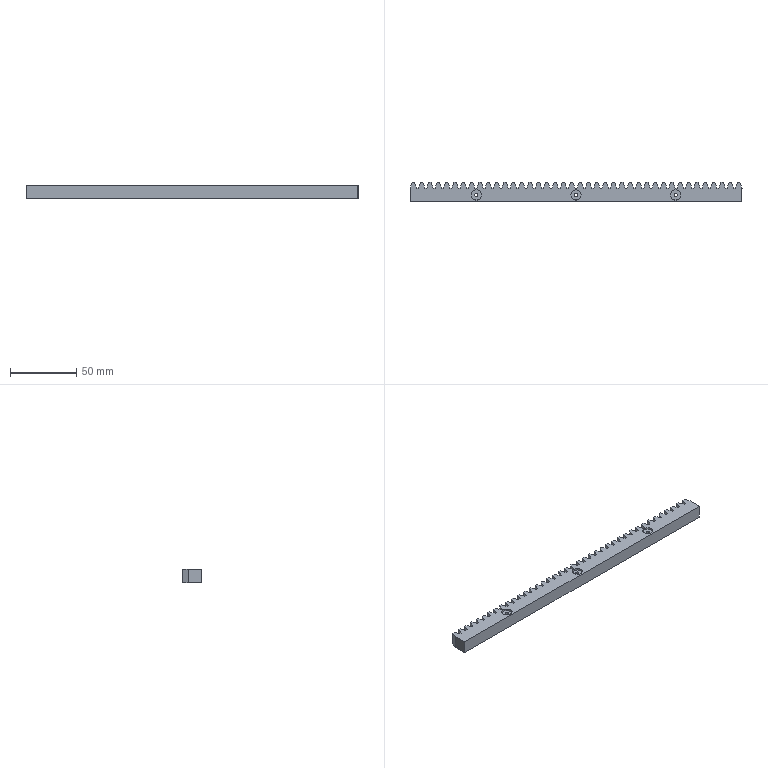Part | SolidWorks | features Boss 1, Extrusion 1, HoleWzd 1, LPattern 1 | 1 solid | 186 faces | box 250.006 x 14.5 x 10 mm | volume 30674 mm3 | plane 168 | cylinder 12 | cone 6 | commonest cylinder face diameters 2.4 x6 7.619 x6